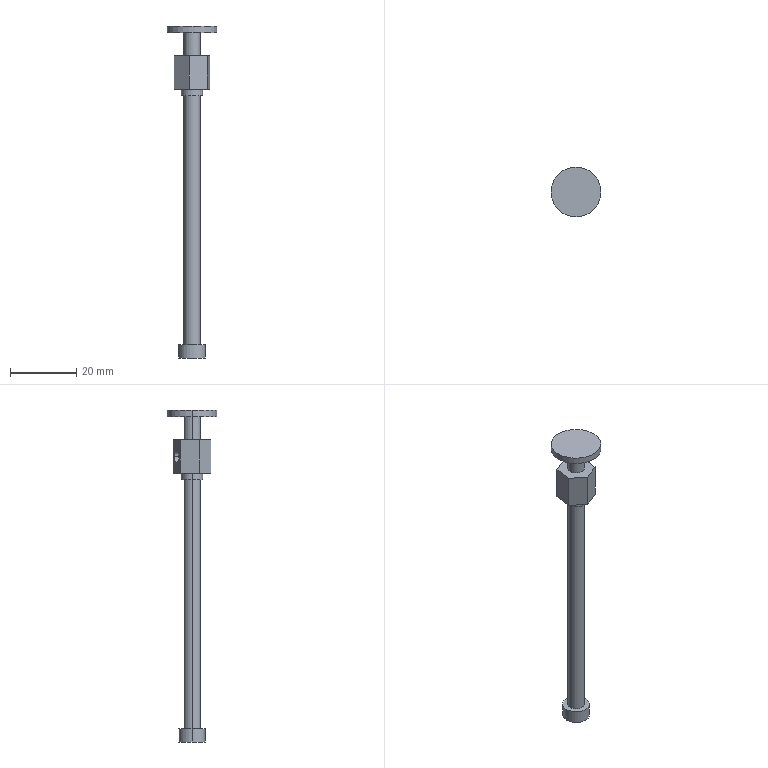Part | SolidWorks | features ICE 5, Extrusion 1 | 1 solid | 26 faces | box 15 x 15 x 100 mm | volume 3078 mm3 | plane 14 | cylinder 12 | commonest cylinder face diameters 5 x4 3.5 x2 6.5 x2 8 x2 15 x2
STEP:
#1=CARTESIAN_POINT('',(21.127,-5.876,86.));
#2=VERTEX_POINT('',#1);
#3=CARTESIAN_POINT('',(17.875,-7.169,86.));
#4=VERTEX_POINT('',#3);
#5=CARTESIAN_POINT('',(19.501,-6.523,86.));
#6=DIRECTION('',(-0.3694,0.9293,0.));
#7=DIRECTION('',(-0.9293,-0.3694,0.));
#8=AXIS2_PLACEMENT_3D('',#5,#6,#7);
#9=CIRCLE('',#8,1.75);
#10=EDGE_CURVE('',#2,#4,#9,.T.);
#11=ORIENTED_EDGE('',*,*,#10,.F.);
#12=CARTESIAN_POINT('',(20.388,-4.018,86.));
#13=VERTEX_POINT('',#12);
#14=CARTESIAN_POINT('',(21.127,-5.876,86.));
#15=DIRECTION('',(-0.3694,0.9293,0.));
#16=VECTOR('',#15,1000.);
#17=LINE('',#14,#16);
#18=EDGE_CURVE('',#2,#13,#17,.T.);
#19=ORIENTED_EDGE('',*,*,#18,.T.);
#20=CARTESIAN_POINT('',(17.136,-5.311,86.));
#21=VERTEX_POINT('',#20);
#22=CARTESIAN_POINT('',(18.762,-4.664,86.));
#23=DIRECTION('',(-0.3694,0.9293,0.));
#24=DIRECTION('',(-0.9293,-0.3694,0.));
#25=AXIS2_PLACEMENT_3D('',#22,#23,#24);
#26=CIRCLE('',#25,1.75);
#27=EDGE_CURVE('',#13,#21,#26,.T.);
#28=ORIENTED_EDGE('',*,*,#27,.T.);
#29=CARTESIAN_POINT('',(17.875,-7.169,86.));
#30=DIRECTION('',(-0.3694,0.9293,0.));
#31=VECTOR('',#30,1000.);
#32=LINE('',#29,#31);
#33=EDGE_CURVE('',#4,#21,#32,.T.);
#34=ORIENTED_EDGE('',*,*,#33,.F.);
#35=EDGE_LOOP('',(#11,#19,#28,#34));
#36=FACE_OUTER_BOUND('',#35,.T.);
#37=CARTESIAN_POINT('',(19.501,-6.523,86.));
#38=DIRECTION('',(-0.3694,0.9293,0.));
#39=DIRECTION('',(-0.9293,-0.3694,0.));
#40=AXIS2_PLACEMENT_3D('',#37,#38,#39);
#41=CYLINDRICAL_SURFACE('',#40,1.75);
#42=ADVANCED_FACE('',(#36),#41,.F.);
#43=CARTESIAN_POINT('',(18.109,-9.311,79.));
#44=VERTEX_POINT('',#43);
#45=CARTESIAN_POINT('',(23.109,-9.311,79.));
#46=VERTEX_POINT('',#45);
#47=CARTESIAN_POINT('',(20.609,-9.311,79.));
#48=DIRECTION('',(0.,0.,-1.));
#49=DIRECTION('',(-1.,0.,0.));
#50=AXIS2_PLACEMENT_3D('',#47,#48,#49);
#51=CIRCLE('',#50,2.5);
#52=EDGE_CURVE('',#44,#46,#51,.T.);
#53=ORIENTED_EDGE('',*,*,#52,.T.);
#54=CARTESIAN_POINT('',(23.109,-9.311,4.));
#55=VERTEX_POINT('',#54);
#56=CARTESIAN_POINT('',(23.109,-9.311,100.));
#57=DIRECTION('',(0.,0.,-1.));
#58=VECTOR('',#57,1000.);
#59=LINE('',#56,#58);
#60=EDGE_CURVE('',#46,#55,#59,.T.);
#61=ORIENTED_EDGE('',*,*,#60,.T.);
#62=CARTESIAN_POINT('',(18.109,-9.311,4.));
#63=VERTEX_POINT('',#62);
#64=CARTESIAN_POINT('',(20.609,-9.311,4.));
#65=DIRECTION('',(0.,0.,-1.));
#66=DIRECTION('',(-1.,0.,0.));
#67=AXIS2_PLACEMENT_3D('',#64,#65,#66);
#68=CIRCLE('',#67,2.5);
#69=EDGE_CURVE('',#63,#55,#68,.T.);
#70=ORIENTED_EDGE('',*,*,#69,.F.);
#71=CARTESIAN_POINT('',(18.109,-9.311,100.));
#72=DIRECTION('',(0.,0.,-1.));
#73=VECTOR('',#72,1000.);
#74=LINE('',#71,#73);
#75=EDGE_CURVE('',#44,#63,#74,.T.);
#76=ORIENTED_EDGE('',*,*,#75,.F.);
#77=EDGE_LOOP('',(#53,#61,#70,#76));
#78=FACE_OUTER_BOUND('',#77,.T.);
#79=CARTESIAN_POINT('',(20.609,-9.311,100.));
#80=DIRECTION('',(0.,0.,-1.));
#81=DIRECTION('',(-1.,0.,0.));
#82=AXIS2_PLACEMENT_3D('',#79,#80,#81);
#83=CYLINDRICAL_SURFACE('',#82,2.5);
#84=ADVANCED_FACE('',(#78),#83,.T.);
#85=CARTESIAN_POINT('',(16.609,-9.311,4.));
#86=VERTEX_POINT('',#85);
#87=CARTESIAN_POINT('',(24.609,-9.311,4.));
#88=VERTEX_POINT('',#87);
#89=CARTESIAN_POINT('',(20.609,-9.311,4.));
#90=DIRECTION('',(0.,0.,-1.));
#91=DIRECTION('',(-1.,0.,0.));
#92=AXIS2_PLACEMENT_3D('',#89,#90,#91);
#93=CIRCLE('',#92,4.);
#94=EDGE_CURVE('',#86,#88,#93,.T.);
#95=ORIENTED_EDGE('',*,*,#94,.T.);
#96=CARTESIAN_POINT('',(24.609,-9.311,0.));
#97=VERTEX_POINT('',#96);
#98=CARTESIAN_POINT('',(24.609,-9.311,4.));
#99=DIRECTION('',(0.,0.,-1.));
#100=VECTOR('',#99,1000.);
#101=LINE('',#98,#100);
#102=EDGE_CURVE('',#88,#97,#101,.T.);
#103=ORIENTED_EDGE('',*,*,#102,.T.);
#104=CARTESIAN_POINT('',(16.609,-9.311,0.));
#105=VERTEX_POINT('',#104);
#106=CARTESIAN_POINT('',(20.609,-9.311,0.));
#107=DIRECTION('',(0.,0.,-1.));
#108=DIRECTION('',(-1.,0.,0.));
#109=AXIS2_PLACEMENT_3D('',#106,#107,#108);
#110=CIRCLE('',#109,4.);
#111=EDGE_CURVE('',#105,#97,#110,.T.);
#112=ORIENTED_EDGE('',*,*,#111,.F.);
#113=CARTESIAN_POINT('',(16.609,-9.311,4.));
#114=DIRECTION('',(0.,0.,-1.));
#115=VECTOR('',#114,1000.);
#116=LINE('',#113,#115);
#117=EDGE_CURVE('',#86,#105,#116,.T.);
#118=ORIENTED_EDGE('',*,*,#117,.F.);
#119=EDGE_LOOP('',(#95,#103,#112,#118));
#120=FACE_OUTER_BOUND('',#119,.T.);
#121=CARTESIAN_POINT('',(20.609,-9.311,4.));
#122=DIRECTION('',(0.,0.,-1.));
#123=DIRECTION('',(-1.,0.,0.));
#124=AXIS2_PLACEMENT_3D('',#121,#122,#123);
#125=CYLINDRICAL_SURFACE('',#124,4.);
#126=ADVANCED_FACE('',(#120),#125,.T.);
#127=CARTESIAN_POINT('',(17.359,-9.311,79.));
#128=VERTEX_POINT('',#127);
#129=CARTESIAN_POINT('',(23.859,-9.311,79.));
#130=VERTEX_POINT('',#129);
#131=CARTESIAN_POINT('',(20.609,-9.311,79.));
#132=DIRECTION('',(0.,0.,-1.));
#133=DIRECTION('',(-1.,0.,0.));
#134=AXIS2_PLACEMENT_3D('',#131,#132,#133);
#135=CIRCLE('',#134,3.25);
#136=EDGE_CURVE('',#128,#130,#135,.T.);
#137=ORIENTED_EDGE('',*,*,#136,.F.);
#138=CARTESIAN_POINT('',(17.359,-9.311,81.));
#139=VERTEX_POINT('',#138);
#140=CARTESIAN_POINT('',(17.359,-9.311,79.));
#141=DIRECTION('',(0.,0.,1.));
#142=VECTOR('',#141,1000.);
#143=LINE('',#140,#142);
#144=EDGE_CURVE('',#128,#139,#143,.T.);
#145=ORIENTED_EDGE('',*,*,#144,.T.);
#146=CARTESIAN_POINT('',(23.859,-9.311,81.));
#147=VERTEX_POINT('',#146);
#148=CARTESIAN_POINT('',(20.609,-9.311,81.));
#149=DIRECTION('',(0.,0.,-1.));
#150=DIRECTION('',(-1.,0.,0.));
#151=AXIS2_PLACEMENT_3D('',#148,#149,#150);
#152=CIRCLE('',#151,3.25);
#153=EDGE_CURVE('',#139,#147,#152,.T.);
#154=ORIENTED_EDGE('',*,*,#153,.T.);
#155=CARTESIAN_POINT('',(23.859,-9.311,79.));
#156=DIRECTION('',(0.,0.,1.));
#157=VECTOR('',#156,1000.);
#158=LINE('',#155,#157);
#159=EDGE_CURVE('',#130,#147,#158,.T.);
#160=ORIENTED_EDGE('',*,*,#159,.F.);
#161=EDGE_LOOP('',(#137,#145,#154,#160));
#162=FACE_OUTER_BOUND('',#161,.T.);
#163=CARTESIAN_POINT('',(20.609,-9.311,79.));
#164=DIRECTION('',(0.,0.,1.));
#165=DIRECTION('',(1.,0.,0.));
#166=AXIS2_PLACEMENT_3D('',#163,#164,#165);
#167=CYLINDRICAL_SURFACE('',#166,3.25);
#168=ADVANCED_FACE('',(#162),#167,.T.);
#169=CARTESIAN_POINT('',(23.109,-9.311,98.));
#170=VERTEX_POINT('',#169);
#171=CARTESIAN_POINT('',(18.109,-9.311,98.));
#172=VERTEX_POINT('',#171);
#173=CARTESIAN_POINT('',(20.609,-9.311,98.));
#174=DIRECTION('',(0.,0.,1.));
#175=DIRECTION('',(1.,0.,0.));
#176=AXIS2_PLACEMENT_3D('',#173,#174,#175);
#177=CIRCLE('',#176,2.5);
#178=EDGE_CURVE('',#170,#172,#177,.T.);
#179=ORIENTED_EDGE('',*,*,#178,.F.);
#180=CARTESIAN_POINT('',(23.109,-9.311,91.));
#181=VERTEX_POINT('',#180);
#182=CARTESIAN_POINT('',(23.109,-9.311,100.));
#183=DIRECTION('',(0.,0.,-1.));
#184=VECTOR('',#183,1000.);
#185=LINE('',#182,#184);
#186=EDGE_CURVE('',#170,#181,#185,.T.);
#187=ORIENTED_EDGE('',*,*,#186,.T.);
#188=CARTESIAN_POINT('',(18.109,-9.311,91.));
#189=VERTEX_POINT('',#188);
#190=CARTESIAN_POINT('',(20.609,-9.311,91.));
#191=DIRECTION('',(0.,0.,-1.));
#192=DIRECTION('',(-1.,0.,0.));
#193=AXIS2_PLACEMENT_3D('',#190,#191,#192);
#194=CIRCLE('',#193,2.5);
#195=EDGE_CURVE('',#189,#181,#194,.T.);
#196=ORIENTED_EDGE('',*,*,#195,.F.);
#197=CARTESIAN_POINT('',(18.109,-9.311,100.));
#198=DIRECTION('',(0.,0.,-1.));
#199=VECTOR('',#198,1000.);
#200=LINE('',#197,#199);
#201=EDGE_CURVE('',#172,#189,#200,.T.);
#202=ORIENTED_EDGE('',*,*,#201,.F.);
#203=EDGE_LOOP('',(#179,#187,#196,#202));
#204=FACE_OUTER_BOUND('',#203,.T.);
#205=CARTESIAN_POINT('',(20.609,-9.311,100.));
#206=DIRECTION('',(0.,0.,-1.));
#207=DIRECTION('',(-1.,0.,0.));
#208=AXIS2_PLACEMENT_3D('',#205,#206,#207);
#209=CYLINDRICAL_SURFACE('',#208,2.5);
#210=ADVANCED_FACE('',(#204),#209,.T.);
#211=CARTESIAN_POINT('',(28.109,-9.311,98.));
#212=VERTEX_POINT('',#211);
#213=CARTESIAN_POINT('',(13.109,-9.311,98.));
#214=VERTEX_POINT('',#213);
#215=CARTESIAN_POINT('',(20.609,-9.311,98.));
#216=DIRECTION('',(0.,0.,1.));
#217=DIRECTION('',(1.,0.,0.));
#218=AXIS2_PLACEMENT_3D('',#215,#216,#217);
#219=CIRCLE('',#218,7.5);
#220=EDGE_CURVE('',#212,#214,#219,.T.);
#221=ORIENTED_EDGE('',*,*,#220,.T.);
#222=CARTESIAN_POINT('',(13.109,-9.311,100.));
#223=VERTEX_POINT('',#222);
#224=CARTESIAN_POINT('',(13.109,-9.311,98.));
#225=DIRECTION('',(0.,0.,1.));
#226=VECTOR('',#225,1000.);
#227=LINE('',#224,#226);
#228=EDGE_CURVE('',#214,#223,#227,.T.);
#229=ORIENTED_EDGE('',*,*,#228,.T.);
#230=CARTESIAN_POINT('',(28.109,-9.311,100.));
#231=VERTEX_POINT('',#230);
#232=CARTESIAN_POINT('',(20.609,-9.311,100.));
#233=DIRECTION('',(0.,0.,1.));
#234=DIRECTION('',(1.,0.,0.));
#235=AXIS2_PLACEMENT_3D('',#232,#233,#234);
#236=CIRCLE('',#235,7.5);
#237=EDGE_CURVE('',#231,#223,#236,.T.);
#238=ORIENTED_EDGE('',*,*,#237,.F.);
#239=CARTESIAN_POINT('',(28.109,-9.311,98.));
#240=DIRECTION('',(0.,0.,1.));
#241=VECTOR('',#240,1000.);
#242=LINE('',#239,#241);
#243=EDGE_CURVE('',#212,#231,#242,.T.);
#244=ORIENTED_EDGE('',*,*,#243,.F.);
#245=EDGE_LOOP('',(#221,#229,#238,#244));
#246=FACE_OUTER_BOUND('',#245,.T.);
#247=CARTESIAN_POINT('',(20.609,-9.311,98.));
#248=DIRECTION('',(0.,0.,1.));
#249=DIRECTION('',(1.,0.,0.));
#250=AXIS2_PLACEMENT_3D('',#247,#248,#249);
#251=CYLINDRICAL_SURFACE('',#250,7.5);
#252=ADVANCED_FACE('',(#246),#251,.T.);
#253=CARTESIAN_POINT('',(15.244,-11.443,91.));
#254=VERTEX_POINT('',#253);
#255=CARTESIAN_POINT('',(16.079,-5.731,91.));
#256=VERTEX_POINT('',#255);
#257=CARTESIAN_POINT('',(15.244,-11.443,91.));
#258=DIRECTION('',(0.1447,0.9895,0.));
#259=VECTOR('',#258,1000.);
#260=LINE('',#257,#259);
#261=EDGE_CURVE('',#254,#256,#260,.T.);
#262=ORIENTED_EDGE('',*,*,#261,.T.);
#263=CARTESIAN_POINT('',(16.079,-5.731,81.));
#264=VERTEX_POINT('',#263);
#265=CARTESIAN_POINT('',(16.079,-5.731,81.));
#266=DIRECTION('',(0.,0.,1.));
#267=VECTOR('',#266,1000.);
#268=LINE('',#265,#267);
#269=EDGE_CURVE('',#264,#256,#268,.T.);
#270=ORIENTED_EDGE('',*,*,#269,.F.);
#271=CARTESIAN_POINT('',(15.244,-11.443,81.));
#272=VERTEX_POINT('',#271);
#273=CARTESIAN_POINT('',(15.244,-11.443,81.));
#274=DIRECTION('',(0.1447,0.9895,0.));
#275=VECTOR('',#274,1000.);
#276=LINE('',#273,#275);
#277=EDGE_CURVE('',#272,#264,#276,.T.);
#278=ORIENTED_EDGE('',*,*,#277,.F.);
#279=CARTESIAN_POINT('',(15.244,-11.443,81.));
#280=DIRECTION('',(0.,0.,1.));
#281=VECTOR('',#280,1000.);
#282=LINE('',#279,#281);
#283=EDGE_CURVE('',#272,#254,#282,.T.);
#284=ORIENTED_EDGE('',*,*,#283,.T.);
#285=EDGE_LOOP('',(#262,#270,#278,#284));
#286=FACE_OUTER_BOUND('',#285,.T.);
#287=CARTESIAN_POINT('',(15.244,-11.443,81.));
#288=DIRECTION('',(0.9895,-0.1447,0.));
#289=DIRECTION('',(0.1447,0.9895,0.));
#290=AXIS2_PLACEMENT_3D('',#287,#288,#289);
#291=PLANE('',#290);
#292=ADVANCED_FACE('',(#286),#291,.F.);
#293=CARTESIAN_POINT('',(18.762,-4.664,86.));
#294=DIRECTION('',(-0.3694,0.9293,0.));
#295=DIRECTION('',(-0.9293,-0.3694,0.));
#296=AXIS2_PLACEMENT_3D('',#293,#294,#295);
#297=CIRCLE('',#296,1.75);
#298=EDGE_CURVE('',#21,#13,#297,.T.);
#299=ORIENTED_EDGE('',*,*,#298,.F.);
#300=ORIENTED_EDGE('',*,*,#27,.F.);
#301=EDGE_LOOP('',(#299,#300));
#302=FACE_BOUND('',#301,.T.);
#303=CARTESIAN_POINT('',(21.445,-3.598,91.));
#304=VERTEX_POINT('',#303);
#305=CARTESIAN_POINT('',(16.079,-5.731,91.));
#306=DIRECTION('',(0.9293,0.3694,0.));
#307=VECTOR('',#306,1000.);
#308=LINE('',#305,#307);
#309=EDGE_CURVE('',#256,#304,#308,.T.);
#310=ORIENTED_EDGE('',*,*,#309,.T.);
#311=CARTESIAN_POINT('',(21.445,-3.598,81.));
#312=VERTEX_POINT('',#311);
#313=CARTESIAN_POINT('',(21.445,-3.598,81.));
#314=DIRECTION('',(0.,0.,1.));
#315=VECTOR('',#314,1000.);
#316=LINE('',#313,#315);
#317=EDGE_CURVE('',#312,#304,#316,.T.);
#318=ORIENTED_EDGE('',*,*,#317,.F.);
#319=CARTESIAN_POINT('',(16.079,-5.731,81.));
#320=DIRECTION('',(0.9293,0.3694,0.));
#321=VECTOR('',#320,1000.);
#322=LINE('',#319,#321);
#323=EDGE_CURVE('',#264,#312,#322,.T.);
#324=ORIENTED_EDGE('',*,*,#323,.F.);
#325=ORIENTED_EDGE('',*,*,#269,.T.);
#326=EDGE_LOOP('',(#310,#318,#324,#325));
#327=FACE_OUTER_BOUND('',#326,.T.);
#328=CARTESIAN_POINT('',(16.079,-5.731,81.));
#329=DIRECTION('',(0.3694,-0.9293,0.));
#330=DIRECTION('',(0.9293,0.3694,0.));
#331=AXIS2_PLACEMENT_3D('',#328,#329,#330);
#332=PLANE('',#331);
#333=ADVANCED_FACE('',(#302,#327),#332,.F.);
#334=CARTESIAN_POINT('',(25.974,-7.178,91.));
#335=VERTEX_POINT('',#334);
#336=CARTESIAN_POINT('',(21.445,-3.598,91.));
#337=DIRECTION('',(0.7845,-0.6201,0.));
#338=VECTOR('',#337,1000.);
#339=LINE('',#336,#338);
#340=EDGE_CURVE('',#304,#335,#339,.T.);
#341=ORIENTED_EDGE('',*,*,#340,.T.);
#342=CARTESIAN_POINT('',(25.974,-7.178,81.));
#343=VERTEX_POINT('',#342);
#344=CARTESIAN_POINT('',(25.974,-7.178,81.));
#345=DIRECTION('',(0.,0.,1.));
#346=VECTOR('',#345,1000.);
#347=LINE('',#344,#346);
#348=EDGE_CURVE('',#343,#335,#347,.T.);
#349=ORIENTED_EDGE('',*,*,#348,.F.);
#350=CARTESIAN_POINT('',(21.445,-3.598,81.));
#351=DIRECTION('',(0.7845,-0.6201,0.));
#352=VECTOR('',#351,1000.);
#353=LINE('',#350,#352);
#354=EDGE_CURVE('',#312,#343,#353,.T.);
#355=ORIENTED_EDGE('',*,*,#354,.F.);
#356=ORIENTED_EDGE('',*,*,#317,.T.);
#357=EDGE_LOOP('',(#341,#349,#355,#356));
#358=FACE_OUTER_BOUND('',#357,.T.);
#359=CARTESIAN_POINT('',(21.445,-3.598,81.));
#360=DIRECTION('',(-0.6201,-0.7845,0.));
#361=DIRECTION('',(0.7845,-0.6201,0.));
#362=AXIS2_PLACEMENT_3D('',#359,#360,#361);
#363=PLANE('',#362);
#364=ADVANCED_FACE('',(#358),#363,.F.);
#365=CARTESIAN_POINT('',(25.139,-12.891,91.));
#366=VERTEX_POINT('',#365);
#367=CARTESIAN_POINT('',(25.974,-7.178,91.));
#368=DIRECTION('',(-0.1447,-0.9895,0.));
#369=VECTOR('',#368,1000.);
#370=LINE('',#367,#369);
#371=EDGE_CURVE('',#335,#366,#370,.T.);
#372=ORIENTED_EDGE('',*,*,#371,.T.);
#373=CARTESIAN_POINT('',(25.139,-12.891,81.));
#374=VERTEX_POINT('',#373);
#375=CARTESIAN_POINT('',(25.139,-12.891,81.));
#376=DIRECTION('',(0.,0.,1.));
#377=VECTOR('',#376,1000.);
#378=LINE('',#375,#377);
#379=EDGE_CURVE('',#374,#366,#378,.T.);
#380=ORIENTED_EDGE('',*,*,#379,.F.);
#381=CARTESIAN_POINT('',(25.974,-7.178,81.));
#382=DIRECTION('',(-0.1447,-0.9895,0.));
#383=VECTOR('',#382,1000.);
#384=LINE('',#381,#383);
#385=EDGE_CURVE('',#343,#374,#384,.T.);
#386=ORIENTED_EDGE('',*,*,#385,.F.);
#387=ORIENTED_EDGE('',*,*,#348,.T.);
#388=EDGE_LOOP('',(#372,#380,#386,#387));
#389=FACE_OUTER_BOUND('',#388,.T.);
#390=CARTESIAN_POINT('',(25.974,-7.178,81.));
#391=DIRECTION('',(-0.9895,0.1447,0.));
#392=DIRECTION('',(-0.1447,-0.9895,0.));
#393=AXIS2_PLACEMENT_3D('',#390,#391,#392);
#394=PLANE('',#393);
#395=ADVANCED_FACE('',(#389),#394,.F.);
#396=CARTESIAN_POINT('',(19.774,-15.023,91.));
#397=VERTEX_POINT('',#396);
#398=CARTESIAN_POINT('',(25.139,-12.891,91.));
#399=DIRECTION('',(-0.9293,-0.3694,0.));
#400=VECTOR('',#399,1000.);
#401=LINE('',#398,#400);
#402=EDGE_CURVE('',#366,#397,#401,.T.);
#403=ORIENTED_EDGE('',*,*,#402,.T.);
#404=CARTESIAN_POINT('',(19.774,-15.023,81.));
#405=VERTEX_POINT('',#404);
#406=CARTESIAN_POINT('',(19.774,-15.023,81.));
#407=DIRECTION('',(0.,0.,1.));
#408=VECTOR('',#407,1000.);
#409=LINE('',#406,#408);
#410=EDGE_CURVE('',#405,#397,#409,.T.);
#411=ORIENTED_EDGE('',*,*,#410,.F.);
#412=CARTESIAN_POINT('',(25.139,-12.891,81.));
#413=DIRECTION('',(-0.9293,-0.3694,0.));
#414=VECTOR('',#413,1000.);
#415=LINE('',#412,#414);
#416=EDGE_CURVE('',#374,#405,#415,.T.);
#417=ORIENTED_EDGE('',*,*,#416,.F.);
#418=ORIENTED_EDGE('',*,*,#379,.T.);
#419=EDGE_LOOP('',(#403,#411,#417,#418));
#420=FACE_OUTER_BOUND('',#419,.T.);
#421=CARTESIAN_POINT('',(25.139,-12.891,81.));
#422=DIRECTION('',(-0.3694,0.9293,0.));
#423=DIRECTION('',(-0.9293,-0.3694,0.));
#424=AXIS2_PLACEMENT_3D('',#421,#422,#423);
#425=PLANE('',#424);
#426=ADVANCED_FACE('',(#420),#425,.F.);
#427=CARTESIAN_POINT('',(19.774,-15.023,91.));
#428=DIRECTION('',(-0.7845,0.6201,0.));
#429=VECTOR('',#428,1000.);
#430=LINE('',#427,#429);
#431=EDGE_CURVE('',#397,#254,#430,.T.);
#432=ORIENTED_EDGE('',*,*,#431,.T.);
#433=ORIENTED_EDGE('',*,*,#283,.F.);
#434=CARTESIAN_POINT('',(19.774,-15.023,81.));
#435=DIRECTION('',(-0.7845,0.6201,0.));
#436=VECTOR('',#435,1000.);
#437=LINE('',#434,#436);
#438=EDGE_CURVE('',#405,#272,#437,.T.);
#439=ORIENTED_EDGE('',*,*,#438,.F.);
#440=ORIENTED_EDGE('',*,*,#410,.T.);
#441=EDGE_LOOP('',(#432,#433,#439,#440));
#442=FACE_OUTER_BOUND('',#441,.T.);
#443=CARTESIAN_POINT('',(19.774,-15.023,81.));
#444=DIRECTION('',(0.6201,0.7845,0.));
#445=DIRECTION('',(-0.7845,0.6201,0.));
#446=AXIS2_PLACEMENT_3D('',#443,#444,#445);
#447=PLANE('',#446);
#448=ADVANCED_FACE('',(#442),#447,.F.);
#449=CARTESIAN_POINT('',(20.609,-9.311,81.));
#450=DIRECTION('',(0.,0.,-1.));
#451=DIRECTION('',(-1.,0.,0.));
#452=AXIS2_PLACEMENT_3D('',#449,#450,#451);
#453=CIRCLE('',#452,3.25);
#454=EDGE_CURVE('',#147,#139,#453,.T.);
#455=ORIENTED_EDGE('',*,*,#454,.F.);
#456=ORIENTED_EDGE('',*,*,#153,.F.);
#457=EDGE_LOOP('',(#455,#456));
#458=FACE_BOUND('',#457,.T.);
#459=ORIENTED_EDGE('',*,*,#277,.T.);
#460=ORIENTED_EDGE('',*,*,#323,.T.);
#461=ORIENTED_EDGE('',*,*,#354,.T.);
#462=ORIENTED_EDGE('',*,*,#385,.T.);
#463=ORIENTED_EDGE('',*,*,#416,.T.);
#464=ORIENTED_EDGE('',*,*,#438,.T.);
#465=EDGE_LOOP('',(#459,#460,#461,#462,#463,#464));
#466=FACE_OUTER_BOUND('',#465,.T.);
#467=CARTESIAN_POINT('',(0.,0.,81.));
#468=DIRECTION('',(0.,0.,-1.));
#469=DIRECTION('',(-1.,0.,0.));
#470=AXIS2_PLACEMENT_3D('',#467,#468,#469);
#471=PLANE('',#470);
#472=ADVANCED_FACE('',(#458,#466),#471,.T.);
#473=ORIENTED_EDGE('',*,*,#195,.T.);
#474=CARTESIAN_POINT('',(20.609,-9.311,91.));
#475=DIRECTION('',(0.,0.,-1.));
#476=DIRECTION('',(-1.,0.,0.));
#477=AXIS2_PLACEMENT_3D('',#474,#475,#476);
#478=CIRCLE('',#477,2.5);
#479=EDGE_CURVE('',#181,#189,#478,.T.);
#480=ORIENTED_EDGE('',*,*,#479,.T.);
#481=EDGE_LOOP('',(#473,#480));
#482=FACE_BOUND('',#481,.T.);
#483=ORIENTED_EDGE('',*,*,#261,.F.);
#484=ORIENTED_EDGE('',*,*,#431,.F.);
#485=ORIENTED_EDGE('',*,*,#402,.F.);
#486=ORIENTED_EDGE('',*,*,#371,.F.);
#487=ORIENTED_EDGE('',*,*,#340,.F.);
#488=ORIENTED_EDGE('',*,*,#309,.F.);
#489=EDGE_LOOP('',(#483,#484,#485,#486,#487,#488));
#490=FACE_OUTER_BOUND('',#489,.T.);
#491=CARTESIAN_POINT('',(0.,0.,91.));
#492=DIRECTION('',(0.,0.,-1.));
#493=DIRECTION('',(-1.,0.,0.));
#494=AXIS2_PLACEMENT_3D('',#491,#492,#493);
#495=PLANE('',#494);
#496=ADVANCED_FACE('',(#482,#490),#495,.F.);
#497=ORIENTED_EDGE('',*,*,#237,.T.);
#498=CARTESIAN_POINT('',(20.609,-9.311,100.));
#499=DIRECTION('',(0.,0.,1.));
#500=DIRECTION('',(1.,0.,0.));
#501=AXIS2_PLACEMENT_3D('',#498,#499,#500);
#502=CIRCLE('',#501,7.5);
#503=EDGE_CURVE('',#223,#231,#502,.T.);
#504=ORIENTED_EDGE('',*,*,#503,.T.);
#505=EDGE_LOOP('',(#497,#504));
#506=FACE_OUTER_BOUND('',#505,.T.);
#507=CARTESIAN_POINT('',(20.609,-9.311,100.));
#508=DIRECTION('',(0.,0.,1.));
#509=DIRECTION('',(1.,0.,0.));
#510=AXIS2_PLACEMENT_3D('',#507,#508,#509);
#511=PLANE('',#510);
#512=ADVANCED_FACE('',(#506),#511,.T.);
#513=ORIENTED_EDGE('',*,*,#228,.F.);
#514=CARTESIAN_POINT('',(20.609,-9.311,98.));
#515=DIRECTION('',(0.,0.,1.));
#516=DIRECTION('',(1.,0.,0.));
#517=AXIS2_PLACEMENT_3D('',#514,#515,#516);
#518=CIRCLE('',#517,7.5);
#519=EDGE_CURVE('',#214,#212,#518,.T.);
#520=ORIENTED_EDGE('',*,*,#519,.T.);
#521=ORIENTED_EDGE('',*,*,#243,.T.);
#522=ORIENTED_EDGE('',*,*,#503,.F.);
#523=EDGE_LOOP('',(#513,#520,#521,#522));
#524=FACE_OUTER_BOUND('',#523,.T.);
#525=CARTESIAN_POINT('',(20.609,-9.311,98.));
#526=DIRECTION('',(0.,0.,1.));
#527=DIRECTION('',(1.,0.,0.));
#528=AXIS2_PLACEMENT_3D('',#525,#526,#527);
#529=CYLINDRICAL_SURFACE('',#528,7.5);
#530=ADVANCED_FACE('',(#524),#529,.T.);
#531=CARTESIAN_POINT('',(20.609,-9.311,98.));
#532=DIRECTION('',(0.,0.,1.));
#533=DIRECTION('',(1.,0.,0.));
#534=AXIS2_PLACEMENT_3D('',#531,#532,#533);
#535=CIRCLE('',#534,2.5);
#536=EDGE_CURVE('',#172,#170,#535,.T.);
#537=ORIENTED_EDGE('',*,*,#536,.T.);
#538=ORIENTED_EDGE('',*,*,#178,.T.);
#539=EDGE_LOOP('',(#537,#538));
#540=FACE_BOUND('',#539,.T.);
#541=ORIENTED_EDGE('',*,*,#220,.F.);
#542=ORIENTED_EDGE('',*,*,#519,.F.);
#543=EDGE_LOOP('',(#541,#542));
#544=FACE_OUTER_BOUND('',#543,.T.);
#545=CARTESIAN_POINT('',(20.609,-9.311,98.));
#546=DIRECTION('',(0.,0.,1.));
#547=DIRECTION('',(1.,0.,0.));
#548=AXIS2_PLACEMENT_3D('',#545,#546,#547);
#549=PLANE('',#548);
#550=ADVANCED_FACE('',(#540,#544),#549,.F.);
#551=ORIENTED_EDGE('',*,*,#186,.F.);
#552=ORIENTED_EDGE('',*,*,#536,.F.);
#553=ORIENTED_EDGE('',*,*,#201,.T.);
#554=ORIENTED_EDGE('',*,*,#479,.F.);
#555=EDGE_LOOP('',(#551,#552,#553,#554));
#556=FACE_OUTER_BOUND('',#555,.T.);
#557=CARTESIAN_POINT('',(20.609,-9.311,100.));
#558=DIRECTION('',(0.,0.,-1.));
#559=DIRECTION('',(-1.,0.,0.));
#560=AXIS2_PLACEMENT_3D('',#557,#558,#559);
#561=CYLINDRICAL_SURFACE('',#560,2.5);
#562=ADVANCED_FACE('',(#556),#561,.T.);
#563=ORIENTED_EDGE('',*,*,#144,.F.);
#564=CARTESIAN_POINT('',(20.609,-9.311,79.));
#565=DIRECTION('',(0.,0.,-1.));
#566=DIRECTION('',(-1.,0.,0.));
#567=AXIS2_PLACEMENT_3D('',#564,#565,#566);
#568=CIRCLE('',#567,3.25);
#569=EDGE_CURVE('',#130,#128,#568,.T.);
#570=ORIENTED_EDGE('',*,*,#569,.F.);
#571=ORIENTED_EDGE('',*,*,#159,.T.);
#572=ORIENTED_EDGE('',*,*,#454,.T.);
#573=EDGE_LOOP('',(#563,#570,#571,#572));
#574=FACE_OUTER_BOUND('',#573,.T.);
#575=CARTESIAN_POINT('',(20.609,-9.311,79.));
#576=DIRECTION('',(0.,0.,1.));
#577=DIRECTION('',(1.,0.,0.));
#578=AXIS2_PLACEMENT_3D('',#575,#576,#577);
#579=CYLINDRICAL_SURFACE('',#578,3.25);
#580=ADVANCED_FACE('',(#574),#579,.T.);
#581=ORIENTED_EDGE('',*,*,#52,.F.);
#582=CARTESIAN_POINT('',(20.609,-9.311,79.));
#583=DIRECTION('',(0.,0.,-1.));
#584=DIRECTION('',(-1.,0.,0.));
#585=AXIS2_PLACEMENT_3D('',#582,#583,#584);
#586=CIRCLE('',#585,2.5);
#587=EDGE_CURVE('',#46,#44,#586,.T.);
#588=ORIENTED_EDGE('',*,*,#587,.F.);
#589=EDGE_LOOP('',(#581,#588));
#590=FACE_BOUND('',#589,.T.);
#591=ORIENTED_EDGE('',*,*,#569,.T.);
#592=ORIENTED_EDGE('',*,*,#136,.T.);
#593=EDGE_LOOP('',(#591,#592));
#594=FACE_OUTER_BOUND('',#593,.T.);
#595=CARTESIAN_POINT('',(20.609,-9.311,79.));
#596=DIRECTION('',(0.,0.,-1.));
#597=DIRECTION('',(-1.,0.,0.));
#598=AXIS2_PLACEMENT_3D('',#595,#596,#597);
#599=PLANE('',#598);
#600=ADVANCED_FACE('',(#590,#594),#599,.T.);
#601=ORIENTED_EDGE('',*,*,#111,.T.);
#602=CARTESIAN_POINT('',(20.609,-9.311,0.));
#603=DIRECTION('',(0.,0.,-1.));
#604=DIRECTION('',(-1.,0.,0.));
#605=AXIS2_PLACEMENT_3D('',#602,#603,#604);
#606=CIRCLE('',#605,4.);
#607=EDGE_CURVE('',#97,#105,#606,.T.);
#608=ORIENTED_EDGE('',*,*,#607,.T.);
#609=EDGE_LOOP('',(#601,#608));
#610=FACE_OUTER_BOUND('',#609,.T.);
#611=CARTESIAN_POINT('',(20.609,-9.311,0.));
#612=DIRECTION('',(0.,0.,1.));
#613=DIRECTION('',(1.,0.,0.));
#614=AXIS2_PLACEMENT_3D('',#611,#612,#613);
#615=PLANE('',#614);
#616=ADVANCED_FACE('',(#610),#615,.F.);
#617=ORIENTED_EDGE('',*,*,#102,.F.);
#618=CARTESIAN_POINT('',(20.609,-9.311,4.));
#619=DIRECTION('',(0.,0.,-1.));
#620=DIRECTION('',(-1.,0.,0.));
#621=AXIS2_PLACEMENT_3D('',#618,#619,#620);
#622=CIRCLE('',#621,4.);
#623=EDGE_CURVE('',#88,#86,#622,.T.);
#624=ORIENTED_EDGE('',*,*,#623,.T.);
#625=ORIENTED_EDGE('',*,*,#117,.T.);
#626=ORIENTED_EDGE('',*,*,#607,.F.);
#627=EDGE_LOOP('',(#617,#624,#625,#626));
#628=FACE_OUTER_BOUND('',#627,.T.);
#629=CARTESIAN_POINT('',(20.609,-9.311,4.));
#630=DIRECTION('',(0.,0.,-1.));
#631=DIRECTION('',(-1.,0.,0.));
#632=AXIS2_PLACEMENT_3D('',#629,#630,#631);
#633=CYLINDRICAL_SURFACE('',#632,4.);
#634=ADVANCED_FACE('',(#628),#633,.T.);
#635=ORIENTED_EDGE('',*,*,#69,.T.);
#636=CARTESIAN_POINT('',(20.609,-9.311,4.));
#637=DIRECTION('',(0.,0.,-1.));
#638=DIRECTION('',(-1.,0.,0.));
#639=AXIS2_PLACEMENT_3D('',#636,#637,#638);
#640=CIRCLE('',#639,2.5);
#641=EDGE_CURVE('',#55,#63,#640,.T.);
#642=ORIENTED_EDGE('',*,*,#641,.T.);
#643=EDGE_LOOP('',(#635,#642));
#644=FACE_BOUND('',#643,.T.);
#645=ORIENTED_EDGE('',*,*,#94,.F.);
#646=ORIENTED_EDGE('',*,*,#623,.F.);
#647=EDGE_LOOP('',(#645,#646));
#648=FACE_OUTER_BOUND('',#647,.T.);
#649=CARTESIAN_POINT('',(20.609,-9.311,4.));
#650=DIRECTION('',(0.,0.,-1.));
#651=DIRECTION('',(-1.,0.,0.));
#652=AXIS2_PLACEMENT_3D('',#649,#650,#651);
#653=PLANE('',#652);
#654=ADVANCED_FACE('',(#644,#648),#653,.F.);
#655=ORIENTED_EDGE('',*,*,#60,.F.);
#656=ORIENTED_EDGE('',*,*,#587,.T.);
#657=ORIENTED_EDGE('',*,*,#75,.T.);
#658=ORIENTED_EDGE('',*,*,#641,.F.);
#659=EDGE_LOOP('',(#655,#656,#657,#658));
#660=FACE_OUTER_BOUND('',#659,.T.);
#661=CARTESIAN_POINT('',(20.609,-9.311,100.));
#662=DIRECTION('',(0.,0.,-1.));
#663=DIRECTION('',(-1.,0.,0.));
#664=AXIS2_PLACEMENT_3D('',#661,#662,#663);
#665=CYLINDRICAL_SURFACE('',#664,2.5);
#666=ADVANCED_FACE('',(#660),#665,.T.);
#667=ORIENTED_EDGE('',*,*,#18,.F.);
#668=CARTESIAN_POINT('',(19.501,-6.523,86.));
#669=DIRECTION('',(-0.3694,0.9293,0.));
#670=DIRECTION('',(-0.9293,-0.3694,0.));
#671=AXIS2_PLACEMENT_3D('',#668,#669,#670);
#672=CIRCLE('',#671,1.75);
#673=EDGE_CURVE('',#4,#2,#672,.T.);
#674=ORIENTED_EDGE('',*,*,#673,.F.);
#675=ORIENTED_EDGE('',*,*,#33,.T.);
#676=ORIENTED_EDGE('',*,*,#298,.T.);
#677=EDGE_LOOP('',(#667,#674,#675,#676));
#678=FACE_OUTER_BOUND('',#677,.T.);
#679=CARTESIAN_POINT('',(19.501,-6.523,86.));
#680=DIRECTION('',(-0.3694,0.9293,0.));
#681=DIRECTION('',(-0.9293,-0.3694,0.));
#682=AXIS2_PLACEMENT_3D('',#679,#680,#681);
#683=CYLINDRICAL_SURFACE('',#682,1.75);
#684=ADVANCED_FACE('',(#678),#683,.F.);
#685=ORIENTED_EDGE('',*,*,#673,.T.);
#686=ORIENTED_EDGE('',*,*,#10,.T.);
#687=EDGE_LOOP('',(#685,#686));
#688=FACE_OUTER_BOUND('',#687,.T.);
#689=CARTESIAN_POINT('',(19.501,-6.523,86.));
#690=DIRECTION('',(-0.3694,0.9293,0.));
#691=DIRECTION('',(-0.9293,-0.3694,0.));
#692=AXIS2_PLACEMENT_3D('',#689,#690,#691);
#693=PLANE('',#692);
#694=ADVANCED_FACE('',(#688),#693,.T.);
#695=CLOSED_SHELL('',(#42,#84,#126,#168,#210,#252,#292,#333,#364,#395,#426,#448,#472,#496,#512,#530,#550,#562,#580,#600,#616,#634,#654,#666,#684,#694));
#696=MANIFOLD_SOLID_BREP('',#695);
#697=CARTESIAN_POINT('',(0.,0.,0.));
#698=DIRECTION('',(0.,0.,1.));
#699=DIRECTION('',(1.,0.,0.));
#700=AXIS2_PLACEMENT_3D('',#697,#698,#699);
#701=(LENGTH_UNIT()NAMED_UNIT(*)SI_UNIT(.MILLI.,.METRE.));
#702=UNCERTAINTY_MEASURE_WITH_UNIT(LENGTH_MEASURE(0.00001),#701,'','');
#703=(NAMED_UNIT(*)PLANE_ANGLE_UNIT()SI_UNIT($,.RADIAN.));
#704=(NAMED_UNIT(*)SI_UNIT($,.STERADIAN.)SOLID_ANGLE_UNIT());
#705=(GEOMETRIC_REPRESENTATION_CONTEXT(3)GLOBAL_UNCERTAINTY_ASSIGNED_CONTEXT((#702))GLOBAL_UNIT_ASSIGNED_CONTEXT((#701,#703,#704))REPRESENTATION_CONTEXT('',''));
#706=ADVANCED_BREP_SHAPE_REPRESENTATION('',(#696,#700),#705);